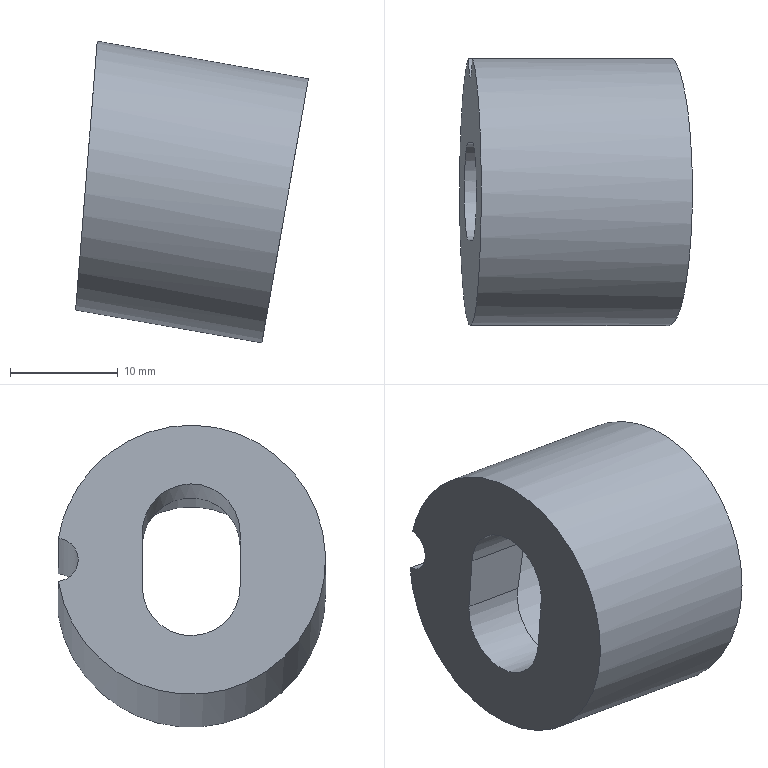Part | NX | features solid 2 | 1 solid | 10 faces | box 21.65 x 24.84 x 28.083 mm | volume 5750 mm3 | cylinder 5 | plane 5 | commonest cylinder face diameters 9.1 x2 4 x1 16.6 x1 25 x1
STEP:
#1=CARTESIAN_POINT('',(-457.49,688.556,-91.424));
#2=VERTEX_POINT('',#1);
#3=CARTESIAN_POINT('',(-438.83,688.556,-94.714));
#4=VERTEX_POINT('',#3);
#5=CARTESIAN_POINT('',(-448.678,688.556,-92.978));
#6=DIRECTION('',(-0.9848,0.,0.1736));
#7=VECTOR('',#6,1000.);
#8=LINE('',#5,#7);
#9=EDGE_CURVE('',#2,#4,#8,.F.);
#10=ORIENTED_EDGE('',*,*,#9,.F.);
#11=CARTESIAN_POINT('',(-457.81,688.556,-95.416));
#12=VERTEX_POINT('',#11);
#13=CARTESIAN_POINT('',(-457.65,676.216,-93.42));
#14=DIRECTION('',(-0.9968,0.,0.08003));
#15=DIRECTION('',(0.08003,0.,0.9968));
#16=AXIS2_PLACEMENT_3D('',#13,#14,#15);
#17=ELLIPSE('',#16,12.556,12.5);
#18=EDGE_CURVE('',#2,#12,#17,.F.);
#19=ORIENTED_EDGE('',*,*,#18,.T.);
#20=CARTESIAN_POINT('',(-439.522,688.556,-98.641));
#21=VERTEX_POINT('',#20);
#22=CARTESIAN_POINT('',(-449.37,688.556,-96.904));
#23=DIRECTION('',(-0.9848,0.,0.1736));
#24=VECTOR('',#23,1000.);
#25=LINE('',#22,#24);
#26=EDGE_CURVE('',#21,#12,#25,.T.);
#27=ORIENTED_EDGE('',*,*,#26,.F.);
#28=CARTESIAN_POINT('',(-439.176,676.216,-96.678));
#29=DIRECTION('',(-0.9848,0.,0.1736));
#30=DIRECTION('',(0.,1.,0.));
#31=AXIS2_PLACEMENT_3D('',#28,#29,#30);
#32=CIRCLE('',#31,12.5);
#33=EDGE_CURVE('',#21,#4,#32,.T.);
#34=ORIENTED_EDGE('',*,*,#33,.T.);
#35=EDGE_LOOP('',(#10,#19,#27,#34));
#36=FACE_BOUND('',#35,.T.);
#37=CARTESIAN_POINT('',(-439.176,676.216,-96.678));
#38=DIRECTION('',(-0.9848,0.,0.1736));
#39=DIRECTION('',(0.,1.,0.));
#40=AXIS2_PLACEMENT_3D('',#37,#38,#39);
#41=CYLINDRICAL_SURFACE('',#40,12.5);
#42=ADVANCED_FACE('',(#36),#41,.T.);
#43=CARTESIAN_POINT('',(-457.65,688.716,-93.42));
#44=DIRECTION('',(-0.9968,0.,0.08003));
#45=DIRECTION('',(0.08003,0.,0.9968));
#46=AXIS2_PLACEMENT_3D('',#43,#44,#45);
#47=ELLIPSE('',#46,2.009,2.);
#48=EDGE_CURVE('',#2,#12,#47,.F.);
#49=ORIENTED_EDGE('',*,*,#48,.F.);
#50=ORIENTED_EDGE('',*,*,#9,.T.);
#51=CARTESIAN_POINT('',(-439.176,688.716,-96.678));
#52=DIRECTION('',(-0.9848,0.,0.1736));
#53=DIRECTION('',(0.,1.,0.));
#54=AXIS2_PLACEMENT_3D('',#51,#52,#53);
#55=CIRCLE('',#54,2.);
#56=EDGE_CURVE('',#21,#4,#55,.T.);
#57=ORIENTED_EDGE('',*,*,#56,.F.);
#58=ORIENTED_EDGE('',*,*,#26,.T.);
#59=EDGE_LOOP('',(#49,#50,#57,#58));
#60=FACE_BOUND('',#59,.T.);
#61=CARTESIAN_POINT('',(-439.176,688.716,-96.678));
#62=DIRECTION('',(-0.9848,0.,0.1736));
#63=DIRECTION('',(0.,1.,0.));
#64=AXIS2_PLACEMENT_3D('',#61,#62,#63);
#65=CYLINDRICAL_SURFACE('',#64,2.);
#66=ADVANCED_FACE('',(#60),#65,.F.);
#67=CARTESIAN_POINT('',(-457.449,671.666,-90.917));
#68=VERTEX_POINT('',#67);
#69=CARTESIAN_POINT('',(-457.851,671.666,-95.923));
#70=VERTEX_POINT('',#69);
#71=CARTESIAN_POINT('',(-457.991,671.666,-97.664));
#72=DIRECTION('',(-0.08003,0.,-0.9968));
#73=VECTOR('',#72,1000.);
#74=LINE('',#71,#73);
#75=EDGE_CURVE('',#68,#70,#74,.T.);
#76=ORIENTED_EDGE('',*,*,#75,.F.);
#77=CARTESIAN_POINT('',(-450.559,671.666,-92.132));
#78=VERTEX_POINT('',#77);
#79=CARTESIAN_POINT('',(-438.742,671.666,-94.216));
#80=DIRECTION('',(-0.9848,0.,0.1736));
#81=VECTOR('',#80,1000.);
#82=LINE('',#79,#81);
#83=EDGE_CURVE('',#78,#68,#82,.T.);
#84=ORIENTED_EDGE('',*,*,#83,.F.);
#85=CARTESIAN_POINT('',(-451.428,671.666,-97.056));
#86=VERTEX_POINT('',#85);
#87=CARTESIAN_POINT('',(-450.993,671.666,-94.594));
#88=DIRECTION('',(0.1736,0.,0.9848));
#89=VECTOR('',#88,1000.);
#90=LINE('',#87,#89);
#91=EDGE_CURVE('',#86,#78,#90,.T.);
#92=ORIENTED_EDGE('',*,*,#91,.F.);
#93=CARTESIAN_POINT('',(-439.61,671.666,-99.14));
#94=DIRECTION('',(-0.9848,0.,0.1736));
#95=VECTOR('',#94,1000.);
#96=LINE('',#93,#95);
#97=EDGE_CURVE('',#86,#70,#96,.T.);
#98=ORIENTED_EDGE('',*,*,#97,.T.);
#99=EDGE_LOOP('',(#76,#84,#92,#98));
#100=FACE_BOUND('',#99,.T.);
#101=CARTESIAN_POINT('',(-439.61,671.666,-99.14));
#102=DIRECTION('',(0.,-1.,0.));
#103=DIRECTION('',(-0.9848,0.,0.1736));
#104=AXIS2_PLACEMENT_3D('',#101,#102,#103);
#105=PLANE('',#104);
#106=ADVANCED_FACE('',(#100),#105,.F.);
#107=CARTESIAN_POINT('',(-457.449,680.766,-90.917));
#108=VERTEX_POINT('',#107);
#109=CARTESIAN_POINT('',(-457.449,676.216,-90.917));
#110=DIRECTION('',(-0.9968,0.,0.08003));
#111=DIRECTION('',(0.08003,0.,0.9968));
#112=AXIS2_PLACEMENT_3D('',#109,#110,#111);
#113=ELLIPSE('',#112,4.57,4.55);
#114=EDGE_CURVE('',#108,#68,#113,.F.);
#115=ORIENTED_EDGE('',*,*,#114,.F.);
#116=CARTESIAN_POINT('',(-450.559,680.766,-92.132));
#117=VERTEX_POINT('',#116);
#118=CARTESIAN_POINT('',(-438.742,680.766,-94.216));
#119=DIRECTION('',(-0.9848,0.,0.1736));
#120=VECTOR('',#119,1000.);
#121=LINE('',#118,#120);
#122=EDGE_CURVE('',#117,#108,#121,.T.);
#123=ORIENTED_EDGE('',*,*,#122,.F.);
#124=CARTESIAN_POINT('',(-450.559,676.216,-92.132));
#125=DIRECTION('',(-0.9848,0.,0.1736));
#126=DIRECTION('',(0.,1.,0.));
#127=AXIS2_PLACEMENT_3D('',#124,#125,#126);
#128=CIRCLE('',#127,4.55);
#129=EDGE_CURVE('',#78,#117,#128,.T.);
#130=ORIENTED_EDGE('',*,*,#129,.F.);
#131=ORIENTED_EDGE('',*,*,#83,.T.);
#132=EDGE_LOOP('',(#115,#123,#130,#131));
#133=FACE_BOUND('',#132,.T.);
#134=CARTESIAN_POINT('',(-438.742,676.216,-94.216));
#135=DIRECTION('',(-0.9848,0.,0.1736));
#136=DIRECTION('',(0.,1.,0.));
#137=AXIS2_PLACEMENT_3D('',#134,#135,#136);
#138=CYLINDRICAL_SURFACE('',#137,4.55);
#139=ADVANCED_FACE('',(#133),#138,.F.);
#140=ORIENTED_EDGE('',*,*,#122,.T.);
#141=CARTESIAN_POINT('',(-457.851,680.766,-95.923));
#142=VERTEX_POINT('',#141);
#143=CARTESIAN_POINT('',(-457.991,680.766,-97.664));
#144=DIRECTION('',(-0.08003,0.,-0.9968));
#145=VECTOR('',#144,1000.);
#146=LINE('',#143,#145);
#147=EDGE_CURVE('',#108,#142,#146,.T.);
#148=ORIENTED_EDGE('',*,*,#147,.T.);
#149=CARTESIAN_POINT('',(-451.428,680.766,-97.056));
#150=VERTEX_POINT('',#149);
#151=CARTESIAN_POINT('',(-439.61,680.766,-99.14));
#152=DIRECTION('',(-0.9848,0.,0.1736));
#153=VECTOR('',#152,1000.);
#154=LINE('',#151,#153);
#155=EDGE_CURVE('',#150,#142,#154,.T.);
#156=ORIENTED_EDGE('',*,*,#155,.F.);
#157=CARTESIAN_POINT('',(-450.993,680.766,-94.594));
#158=DIRECTION('',(0.1736,0.,0.9848));
#159=VECTOR('',#158,1000.);
#160=LINE('',#157,#159);
#161=EDGE_CURVE('',#150,#117,#160,.T.);
#162=ORIENTED_EDGE('',*,*,#161,.T.);
#163=EDGE_LOOP('',(#140,#148,#156,#162));
#164=FACE_BOUND('',#163,.T.);
#165=CARTESIAN_POINT('',(-439.61,680.766,-99.14));
#166=DIRECTION('',(0.,-1.,0.));
#167=DIRECTION('',(-0.9848,0.,0.1736));
#168=AXIS2_PLACEMENT_3D('',#165,#166,#167);
#169=PLANE('',#168);
#170=ADVANCED_FACE('',(#164),#169,.T.);
#171=CARTESIAN_POINT('',(-457.851,676.216,-95.923));
#172=DIRECTION('',(-0.9968,0.,0.08003));
#173=DIRECTION('',(0.08003,0.,0.9968));
#174=AXIS2_PLACEMENT_3D('',#171,#172,#173);
#175=ELLIPSE('',#174,4.57,4.55);
#176=EDGE_CURVE('',#70,#142,#175,.F.);
#177=ORIENTED_EDGE('',*,*,#176,.F.);
#178=ORIENTED_EDGE('',*,*,#97,.F.);
#179=CARTESIAN_POINT('',(-451.428,676.216,-97.056));
#180=DIRECTION('',(-0.9848,0.,0.1736));
#181=DIRECTION('',(0.,1.,0.));
#182=AXIS2_PLACEMENT_3D('',#179,#180,#181);
#183=CIRCLE('',#182,4.55);
#184=EDGE_CURVE('',#150,#86,#183,.T.);
#185=ORIENTED_EDGE('',*,*,#184,.F.);
#186=ORIENTED_EDGE('',*,*,#155,.T.);
#187=EDGE_LOOP('',(#177,#178,#185,#186));
#188=FACE_BOUND('',#187,.T.);
#189=CARTESIAN_POINT('',(-439.61,676.216,-99.14));
#190=DIRECTION('',(-0.9848,0.,0.1736));
#191=DIRECTION('',(0.,1.,0.));
#192=AXIS2_PLACEMENT_3D('',#189,#190,#191);
#193=CYLINDRICAL_SURFACE('',#192,4.55);
#194=ADVANCED_FACE('',(#188),#193,.F.);
#195=CARTESIAN_POINT('',(-439.176,684.516,-96.678));
#196=VERTEX_POINT('',#195);
#197=CARTESIAN_POINT('',(-439.176,676.216,-96.678));
#198=DIRECTION('',(-0.9848,0.,0.1736));
#199=DIRECTION('',(0.,1.,0.));
#200=AXIS2_PLACEMENT_3D('',#197,#198,#199);
#201=CIRCLE('',#200,8.3);
#202=EDGE_CURVE('',#196,#196,#201,.T.);
#203=ORIENTED_EDGE('',*,*,#202,.T.);
#204=EDGE_LOOP('',(#203));
#205=FACE_BOUND('',#204,.T.);
#206=ORIENTED_EDGE('',*,*,#33,.F.);
#207=ORIENTED_EDGE('',*,*,#56,.T.);
#208=EDGE_LOOP('',(#206,#207));
#209=FACE_BOUND('',#208,.T.);
#210=CARTESIAN_POINT('',(-439.176,676.216,-96.678));
#211=DIRECTION('',(-0.9848,0.,0.1736));
#212=DIRECTION('',(0.,1.,0.));
#213=AXIS2_PLACEMENT_3D('',#210,#211,#212);
#214=PLANE('',#213);
#215=ADVANCED_FACE('',(#205,#209),#214,.F.);
#216=ORIENTED_EDGE('',*,*,#202,.F.);
#217=EDGE_LOOP('',(#216));
#218=FACE_BOUND('',#217,.T.);
#219=CARTESIAN_POINT('',(-450.993,684.516,-94.594));
#220=VERTEX_POINT('',#219);
#221=CARTESIAN_POINT('',(-450.993,676.216,-94.594));
#222=DIRECTION('',(-0.9848,0.,0.1736));
#223=DIRECTION('',(0.,1.,0.));
#224=AXIS2_PLACEMENT_3D('',#221,#222,#223);
#225=CIRCLE('',#224,8.3);
#226=EDGE_CURVE('',#220,#220,#225,.T.);
#227=ORIENTED_EDGE('',*,*,#226,.T.);
#228=EDGE_LOOP('',(#227));
#229=FACE_BOUND('',#228,.T.);
#230=CARTESIAN_POINT('',(-439.176,676.216,-96.678));
#231=DIRECTION('',(-0.9848,0.,0.1736));
#232=DIRECTION('',(0.,1.,0.));
#233=AXIS2_PLACEMENT_3D('',#230,#231,#232);
#234=CYLINDRICAL_SURFACE('',#233,8.3);
#235=ADVANCED_FACE('',(#218,#229),#234,.F.);
#236=ORIENTED_EDGE('',*,*,#184,.T.);
#237=ORIENTED_EDGE('',*,*,#91,.T.);
#238=ORIENTED_EDGE('',*,*,#129,.T.);
#239=ORIENTED_EDGE('',*,*,#161,.F.);
#240=EDGE_LOOP('',(#236,#237,#238,#239));
#241=FACE_BOUND('',#240,.T.);
#242=ORIENTED_EDGE('',*,*,#226,.F.);
#243=EDGE_LOOP('',(#242));
#244=FACE_BOUND('',#243,.T.);
#245=CARTESIAN_POINT('',(-450.993,676.216,-94.594));
#246=DIRECTION('',(-0.9848,0.,0.1736));
#247=DIRECTION('',(0.,1.,0.));
#248=AXIS2_PLACEMENT_3D('',#245,#246,#247);
#249=PLANE('',#248);
#250=ADVANCED_FACE('',(#241,#244),#249,.F.);
#251=ORIENTED_EDGE('',*,*,#18,.F.);
#252=ORIENTED_EDGE('',*,*,#48,.T.);
#253=EDGE_LOOP('',(#251,#252));
#254=FACE_BOUND('',#253,.T.);
#255=ORIENTED_EDGE('',*,*,#114,.T.);
#256=ORIENTED_EDGE('',*,*,#75,.T.);
#257=ORIENTED_EDGE('',*,*,#176,.T.);
#258=ORIENTED_EDGE('',*,*,#147,.F.);
#259=EDGE_LOOP('',(#255,#256,#257,#258));
#260=FACE_BOUND('',#259,.T.);
#261=CARTESIAN_POINT('',(-448.537,482.597,20.085));
#262=DIRECTION('',(-0.9968,0.,0.08003));
#263=DIRECTION('',(-0.08003,0.,-0.9968));
#264=AXIS2_PLACEMENT_3D('',#261,#262,#263);
#265=PLANE('',#264);
#266=ADVANCED_FACE('',(#254,#260),#265,.T.);
#267=CLOSED_SHELL('',(#42,#66,#106,#139,#170,#194,#215,#235,#250,#266));
#268=MANIFOLD_SOLID_BREP('',#267);
#269=(LENGTH_UNIT()NAMED_UNIT(*)SI_UNIT(.MILLI.,.METRE.));
#270=UNCERTAINTY_MEASURE_WITH_UNIT(LENGTH_MEASURE(0.00001),#269,'','');
#271=(NAMED_UNIT(*)PLANE_ANGLE_UNIT()SI_UNIT($,.RADIAN.));
#272=(NAMED_UNIT(*)SI_UNIT($,.STERADIAN.)SOLID_ANGLE_UNIT());
#273=(GEOMETRIC_REPRESENTATION_CONTEXT(3)GLOBAL_UNCERTAINTY_ASSIGNED_CONTEXT((#270))GLOBAL_UNIT_ASSIGNED_CONTEXT((#269,#271,#272))REPRESENTATION_CONTEXT('',''));
#274=ADVANCED_BREP_SHAPE_REPRESENTATION('',(#268),#273);